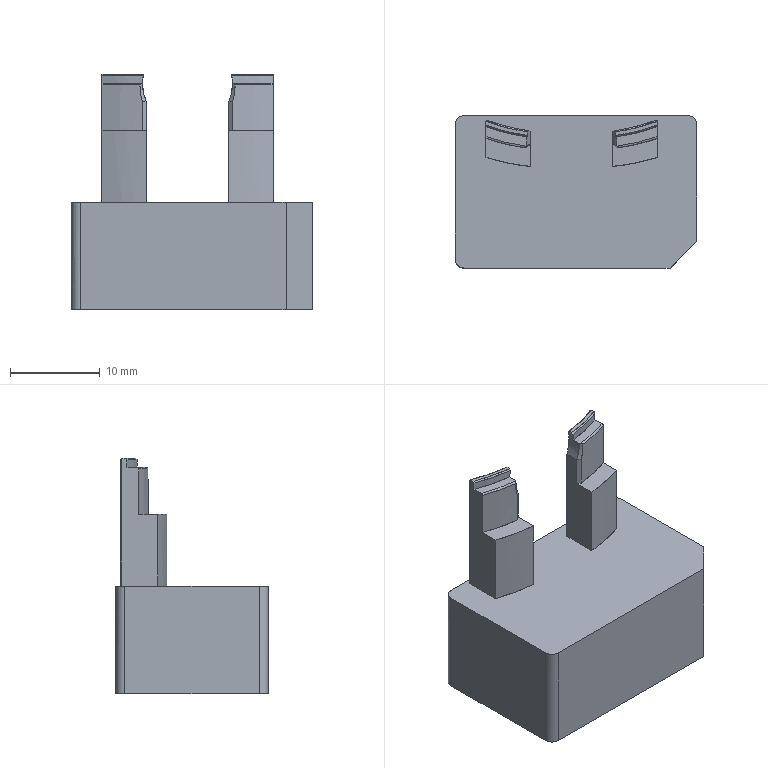NC program | PowerMill | posted by the shop | part box 27 x 17 x 26.255 mm
Lines 1 to 1491 of 169183:
%
G40 G49 G17 G80
( TOOL ID   D10C_1_1_1 )
( TOOL DIA. 10. TIP RAD 0 LENGTH 81.72 )
( Z = -.065 )
T1 M6
T15
G91 G28 Z0
G0 G90 G54
M08
S8000 M3
G0 X0 Y0 M8
G43 Z10.2 H1
X21.28 Y11.28
Z1.135
G1 Z-.065 F6000
X16.28 F10000
X-16.28
Y5.64
X16.28
Y0
X-16.28
Y-5.64
X16.28
Y-11.28
X-16.28
X-21.28
G0 Z10.2
X-.501 Y2.234
Z9.885
X-23.108 Y2.522
Z.76
G1 Z-.44 F6000
X-22.58 F10000
G3 X-17.833 Y7.269 I0 J4.748
G1 Y14.747
G2 X-16.833 Y15.747 I1. J0
G1 X15.832
G2 X16.832 Y14.747 I0 J-1.
G1 Y-10.28
G2 X15.832 Y-11.28 I-1. J0
G1 X-.501
Y-5.336
X-11.502
G2 X-11.889 Y-4.949 I0 J.387
G1 Y-4.312
G2 X-11.528 Y-4.044 I.28 J0
G1 X-11.418 Y-4.077
X-9.556 Y-4.534
X-9.269 Y-4.594
X-8.456 Y-4.751
X-7.639 Y-4.886
X-7.129 Y-4.964
X-6.703 Y-5.019
X-6.274 Y-5.057
X-6.168 Y-5.064
G3 X-3.449 Y-4.906 I.725 J11.016
G1 X-3.329 Y-4.884
G3 X-1.802 Y-4.477 I-1.811 J9.863
G1 X-1.62 Y-4.412
X-1.392 Y-4.327
X-1.167 Y-4.232
X-.975 Y-4.146
G2 X-.025 Y-4.146 I.475 J-1.064
G1 X.167 Y-4.232
X.39 Y-4.326
X.616 Y-4.411
X.799 Y-4.476
G3 X2.328 Y-4.884 I3.341 J9.454
G1 X2.448 Y-4.906
G3 X5.138 Y-5.066 I1.994 J10.86
G1 X5.232 Y-5.06
X5.64 Y-5.025
X6.047 Y-4.972
X7.251 Y-4.788
X9.342 Y-4.355
X10.523 Y-4.035
G2 X10.888 Y-4.314 I.076 J-.279
G1 Y-4.949
G2 X10.501 Y-5.336 I-.387 J0
G1 X-.501
Y-11.28
X-16.833
G2 X-17.833 Y-10.28 I0 J1.
G1 Y7.269
X-15.332 Y7.261
X-15.329 Y8.034
X-15.249 Y8.808
X-15.053 Y9.581
X-14.724 Y10.354
X-14.422 Y10.863
X-14.232 Y11.128
X-13.649 Y11.779
X-12.875 Y12.387
X-12.374 Y12.675
X-12.102 Y12.802
X-11.328 Y13.071
X-10.555 Y13.217
X-9.782 Y13.248
X-9.008 Y13.167
X-8.235 Y12.969
X-7.461 Y12.698
X-6.688 Y12.468
X-5.914 Y12.282
X-4.368 Y11.988
X-4.013 Y11.901
X-3.594 Y11.764
X-2.821 Y11.4
X-2.395 Y11.128
X-2.047 Y10.859
X-1.525 Y10.354
X-1.274 Y10.054
X-.947 Y9.581
G3 X-.053 Y9.581 I.447 J.224
G1 X.273 Y10.053
X.525 Y10.354
X1.046 Y10.859
X1.395 Y11.128
X1.82 Y11.4
X2.593 Y11.764
X3.013 Y11.901
X4.14 Y12.133
X5.687 Y12.46
X7.234 Y12.969
X8.007 Y13.167
X8.781 Y13.248
X9.554 Y13.217
X10.327 Y13.072
X11.101 Y12.803
X11.374 Y12.675
X11.874 Y12.388
X12.515 Y11.901
X13.232 Y11.128
X13.421 Y10.864
X13.724 Y10.354
X14.053 Y9.581
X14.249 Y8.808
X14.329 Y8.034
X14.332 Y7.261
X14.272 Y6.487
X14.195 Y6.068
X14.09 Y5.714
X13.788 Y4.94
X13.329 Y4.167
X12.64 Y3.394
X11.874 Y2.802
X11.563 Y2.62
X11.101 Y2.398
X9.554 Y1.862
X8.007 Y1.436
X6.269 Y1.073
X4.913 Y.875
X4.14 Y.864
X3.367 Y.968
X2.95 Y1.073
X2.593 Y1.193
X1.82 Y1.558
X1.372 Y1.847
X1.046 Y2.1
X.512 Y2.62
X.273 Y2.908
X-.061 Y3.394
G3 X-.939 Y3.394 I-.439 J-.238
G1 X-1.274 Y2.907
X-1.512 Y2.62
X-2.047 Y2.099
X-2.372 Y1.847
X-2.821 Y1.557
X-3.594 Y1.193
X-3.95 Y1.073
X-4.368 Y.968
X-5.141 Y.864
X-5.914 Y.876
X-6.688 Y.978
X-8.235 Y1.26
X-9.782 Y1.636
X-11.328 Y2.114
X-12.102 Y2.398
X-12.561 Y2.62
X-12.875 Y2.802
X-13.649 Y3.399
X-14.325 Y4.167
X-14.789 Y4.94
X-15.091 Y5.714
X-15.196 Y6.072
X-15.272 Y6.487
X-15.332 Y7.261
X-17.833 Y7.269
G0 Z3.435
G1 X-23.108 Y2.522
G0 Z.435
G1 Z-.765 F6000
X-22.58 F10000
G3 X-17.833 Y7.269 I0 J4.748
G1 Y14.747
G2 X-16.833 Y15.747 I1. J0
G1 X15.832
G2 X16.832 Y14.747 I0 J-1.
G1 Y-10.28
G2 X15.832 Y-11.28 I-1. J0
G1 X-.501
Y-5.336
X-11.502
G2 X-11.889 Y-4.949 I0 J.387
G1 Y-4.312
G2 X-11.528 Y-4.044 I.28 J0
G1 X-11.418 Y-4.077
X-9.556 Y-4.534
X-9.269 Y-4.594
X-8.456 Y-4.751
X-7.639 Y-4.886
X-7.129 Y-4.964
X-6.702 Y-5.019
X-6.273 Y-5.057
X-6.167 Y-5.064
G3 X-3.45 Y-4.906 I.724 J11.015
G1 X-3.33 Y-4.884
G3 X-1.802 Y-4.477 I-1.81 J9.864
G1 X-1.619 Y-4.413
X-1.363 Y-4.315
X-1.111 Y-4.207
X-.994 Y-4.153
G2 X-.006 Y-4.153 I.494 J-1.076
G1 X.111 Y-4.207
X.361 Y-4.315
X.616 Y-4.411
X.799 Y-4.476
G3 X2.329 Y-4.884 I3.341 J9.455
G1 X2.449 Y-4.906
G3 X5.137 Y-5.066 I1.993 J10.86
G1 X5.231 Y-5.06
X5.64 Y-5.025
X6.047 Y-4.972
X7.251 Y-4.788
X9.342 Y-4.355
X10.523 Y-4.035
G2 X10.888 Y-4.314 I.076 J-.279
G1 Y-4.949
G2 X10.501 Y-5.336 I-.387 J0
G1 X-.501
Y-11.28
X-16.833
G2 X-17.833 Y-10.28 I0 J1.
G1 Y7.269
X-15.332 Y7.261
X-15.329 Y8.034
X-15.249 Y8.808
X-15.053 Y9.581
X-14.724 Y10.354
X-14.422 Y10.863
X-14.232 Y11.128
X-13.649 Y11.779
X-12.875 Y12.387
X-12.374 Y12.675
X-12.102 Y12.802
X-11.328 Y13.071
X-10.555 Y13.217
X-9.782 Y13.248
X-9.008 Y13.167
X-8.235 Y12.969
X-7.396 Y12.678
X-7.179 Y12.614
X-6.688 Y12.469
X-5.914 Y12.288
X-5.451 Y12.194
X-4.368 Y11.988
X-4.014 Y11.902
X-4.012 Y11.901
X-3.594 Y11.764
X-2.821 Y11.4
X-2.395 Y11.128
X-2.047 Y10.859
X-1.525 Y10.354
X-1.274 Y10.054
X-.947 Y9.581
G3 X-.053 Y9.581 I.447 J.224
G1 X.273 Y10.053
X.525 Y10.354
X1.046 Y10.859
X1.395 Y11.128
X1.82 Y11.4
X2.593 Y11.764
X3.013 Y11.901
X4.14 Y12.133
X5.687 Y12.468
X5.958 Y12.549
X7.23 Y12.968
X7.234 Y12.969
X8.007 Y13.167
X8.781 Y13.248
X9.554 Y13.217
X10.327 Y13.072
X11.101 Y12.803
X11.374 Y12.675
X11.874 Y12.388
X12.515 Y11.901
X13.232 Y11.128
X13.421 Y10.864
X13.724 Y10.354
X14.053 Y9.581
X14.249 Y8.808
X14.329 Y8.034
X14.332 Y7.261
X14.276 Y6.487
X14.195 Y6.068
X14.095 Y5.714
X13.793 Y4.94
X13.334 Y4.167
X12.648 Y3.398
X11.874 Y2.802
X11.567 Y2.62
X11.101 Y2.398
X9.554 Y1.862
X8.007 Y1.436
X6.269 Y1.073
X4.913 Y.875
X4.14 Y.864
X3.367 Y.968
X2.95 Y1.073
X2.593 Y1.193
X1.82 Y1.558
X1.372 Y1.847
X1.046 Y2.1
X.512 Y2.62
X.273 Y2.908
X-.061 Y3.394
G3 X-.939 Y3.394 I-.439 J-.239
G1 X-1.274 Y2.907
X-1.512 Y2.62
X-2.047 Y2.099
X-2.372 Y1.847
X-2.821 Y1.557
X-3.594 Y1.193
X-3.95 Y1.073
X-4.368 Y.968
X-5.141 Y.864
X-5.914 Y.876
X-6.688 Y.978
X-8.235 Y1.26
X-9.782 Y1.636
X-11.328 Y2.114
X-12.102 Y2.398
X-12.564 Y2.62
X-12.875 Y2.802
X-13.643 Y3.394
X-13.646 Y3.396
X-13.649 Y3.399
X-13.755 Y3.519
X-14.33 Y4.167
X-14.794 Y4.94
X-15.096 Y5.714
X-15.196 Y6.072
X-15.277 Y6.487
X-15.332 Y7.261
X-17.833 Y7.269
G0 Z3.11
G1 X-23.108 Y2.522
G0 Z.11
G1 Z-1.09 F6000
X-22.58 F10000
G3 X-17.833 Y7.269 I0 J4.748
G1 Y14.747
G2 X-16.833 Y15.747 I1. J0
G1 X15.832
G2 X16.832 Y14.747 I0 J-1.
G1 Y-10.28
G2 X15.832 Y-11.28 I-1. J0
G1 X-.501
Y-5.336
X-11.502
G2 X-11.889 Y-4.949 I0 J.387
G1 Y-4.312
G2 X-11.528 Y-4.044 I.28 J0
G1 X-11.418 Y-4.077
X-9.556 Y-4.534
X-9.269 Y-4.594
X-8.456 Y-4.751
X-7.638 Y-4.886
X-7.129 Y-4.964
X-6.702 Y-5.019
X-6.273 Y-5.057
X-6.166 Y-5.064
G3 X-3.451 Y-4.906 I.724 J11.015
G1 X-3.331 Y-4.884
G3 X-1.802 Y-4.477 I-1.809 J9.864
G1 X-1.619 Y-4.413
X-1.363 Y-4.315
X-1.111 Y-4.207
X-.994 Y-4.153
G2 X-.006 Y-4.153 I.494 J-1.076
G1 X.111 Y-4.207
X.361 Y-4.315
X.616 Y-4.411
X.799 Y-4.476
G3 X2.331 Y-4.884 I3.341 J9.455
G1 X2.451 Y-4.906
G3 X5.136 Y-5.066 I1.992 J10.859
G1 X5.231 Y-5.06
X5.64 Y-5.025
X6.047 Y-4.972
X7.251 Y-4.788
X9.342 Y-4.355
X10.523 Y-4.035
G2 X10.888 Y-4.314 I.076 J-.279
G1 Y-4.949
G2 X10.501 Y-5.336 I-.387 J0
G1 X-.501
Y-11.28
X-16.833
G2 X-17.833 Y-10.28 I0 J1.
G1 Y6.806
X-15.313 Y6.971
X-15.332 Y7.261
X-15.329 Y8.034
X-15.249 Y8.808
X-15.053 Y9.581
X-14.724 Y10.354
X-14.422 Y10.863
X-14.232 Y11.128
X-13.649 Y11.779
X-12.875 Y12.387
X-12.374 Y12.675
X-12.102 Y12.802
X-11.328 Y13.071
X-10.555 Y13.217
X-9.782 Y13.248
X-9.008 Y13.167
X-8.235 Y12.969
X-7.374 Y12.675
X-6.688 Y12.471
X-5.914 Y12.29
X-5.354 Y12.175
X-4.368 Y11.988
X-4.015 Y11.902
X-4.012 Y11.901
X-3.594 Y11.764
X-2.821 Y11.4
X-2.395 Y11.128
X-2.047 Y10.859
X-1.525 Y10.354
X-1.274 Y10.054
X-.947 Y9.581
G3 X-.053 Y9.581 I.447 J.224
G1 X.273 Y10.053
X.525 Y10.354
X1.046 Y10.859
X1.395 Y11.128
X1.82 Y11.4
X2.593 Y11.764
X3.013 Y11.901
X4.14 Y12.133
X5.687 Y12.471
X6.016 Y12.568
X7.226 Y12.966
X7.234 Y12.969
X8.007 Y13.167
X8.781 Y13.248
X9.554 Y13.217
X10.327 Y13.072
X11.101 Y12.803
X11.374 Y12.675
X11.874 Y12.388
X12.515 Y11.901
X13.232 Y11.128
X13.421 Y10.864
X13.724 Y10.354
X14.053 Y9.581
X14.249 Y8.808
X14.329 Y8.034
X14.332 Y7.261
X14.28 Y6.487
X14.255 Y6.378
X14.195 Y6.068
X14.123 Y5.813
X14.099 Y5.714
X13.797 Y4.94
X13.338 Y4.167
X12.647 Y3.394
X11.874 Y2.802
X11.571 Y2.62
X11.101 Y2.398
X9.554 Y1.862
X8.007 Y1.436
X6.269 Y1.073
X4.913 Y.875
X4.14 Y.864
X3.367 Y.968
X2.95 Y1.073
X2.593 Y1.193
X1.82 Y1.558
X1.372 Y1.847
X1.046 Y2.1
X.512 Y2.62
X.273 Y2.908
X-.061 Y3.394
G3 X-.939 Y3.394 I-.439 J-.239
G1 X-1.274 Y2.907
X-1.512 Y2.62
X-2.047 Y2.099
X-2.372 Y1.847
X-2.821 Y1.557
X-3.594 Y1.193
X-3.95 Y1.073
X-4.368 Y.968
X-5.141 Y.864
X-5.914 Y.876
X-6.688 Y.978
X-8.235 Y1.26
X-9.782 Y1.636
X-11.328 Y2.114
X-12.102 Y2.398
X-12.568 Y2.62
X-12.875 Y2.802
X-12.979 Y2.882
X-13.643 Y3.394
X-13.645 Y3.396
X-13.649 Y3.399
X-14.335 Y4.167
X-14.798 Y4.94
X-15.1 Y5.714
X-15.125 Y5.821
X-15.196 Y6.072
X-15.252 Y6.363
X-15.281 Y6.487
X-15.313 Y6.971
X-17.833 Y6.806
Y7.269
G0 Z2.735
G1 X-23.108 Y2.522
G0 Z-.265
G1 Z-1.465 F6000
X-22.58 F10000
G3 X-17.833 Y7.269 I0 J4.748
G1 Y14.747
G2 X-16.833 Y15.747 I1. J0
G1 X15.832
G2 X16.832 Y14.747 I0 J-1.
G1 Y-5.393
X11.752 Y-5.243
G2 X11.308 Y-5.956 I-.835 J.025
G1 X11.191 Y-6.018
X10.983 Y-6.097
X10.763 Y-6.124
X-11.764
X-11.975 Y-6.099
X-12.175 Y-6.027
X-12.288 Y-5.97
G2 X-11.603 Y-4.427 I.38 J.755
G1 X-11.306 Y-4.542
G3 X-1.746 Y-4.671 I4.954 J12.815
G1 X-1.183 Y-4.471
G2 X.087 Y-4.447 I.67 J-1.884
G1 X1.604 Y-4.924
G3 X10.315 Y-4.562 I3.853 J12.262
G1 X10.601 Y-4.445
G2 X11.752 Y-5.243 I.316 J-.773
G1 X16.832 Y-5.393
Y-10.28
G2 X15.832 Y-11.28 I-1. J0
G1 X-16.833
G2 X-17.833 Y-10.28 I0 J1.
G1 Y5.711
X-15.327 Y5.714
X-15.328 Y7.209
X-15.332 Y7.261
X-15.329 Y8.022
Y8.034
X-15.249 Y8.808
X-15.053 Y9.581
X-14.724 Y10.354
X-14.422 Y10.863
X-14.232 Y11.128
X-13.649 Y11.779
X-12.875 Y12.387
X-12.374 Y12.675
X-12.102 Y12.802
X-11.328 Y13.071
X-10.555 Y13.217
X-9.782 Y13.248
X-9.008 Y13.167
X-8.235 Y12.969
X-7.374 Y12.675
X-6.688 Y12.474
X-5.914 Y12.29
X-5.331 Y12.171
X-4.368 Y11.988
X-4.017 Y11.902
X-4.012 Y11.901
X-3.594 Y11.764
X-2.821 Y11.4
X-2.395 Y11.128
X-2.047 Y10.859
X-1.525 Y10.354
X-1.274 Y10.054
X-.947 Y9.581
G3 X-.053 Y9.581 I.447 J.224
G1 X.273 Y10.053
X.525 Y10.354
X1.046 Y10.859
X1.395 Y11.128
X1.82 Y11.4
X2.593 Y11.764
X3.013 Y11.901
X4.14 Y12.133
X5.687 Y12.473
X6.087 Y12.591
X7.219 Y12.964
X7.234 Y12.969
X8.007 Y13.167
X8.781 Y13.248
X9.554 Y13.217
X10.327 Y13.072
X11.101 Y12.803
X11.374 Y12.675
X11.874 Y12.388
X12.515 Y11.901
X13.232 Y11.128
X13.421 Y10.864
X13.724 Y10.354
X14.053 Y9.581
X14.249 Y8.808
X14.329 Y8.034
Y8.022
X14.332 Y7.261
X14.328 Y7.211
X14.327 Y5.714
X14.236 Y4.94
X14.024 Y4.167
X13.675 Y3.394
X13.421 Y2.98
X13.154 Y2.62
X12.648 Y2.078
X12.382 Y1.847
X11.874 Y1.482
X11.101 Y1.078
X10.327 Y.804
X9.554 Y.564
X8.59 Y.3
X7.234 Y-.01
X5.687 Y-.276
X4.913 Y-.343
X4.14 Y-.307
X3.367 Y-.15
X2.593 Y.138
X2.277 Y.3
X1.82 Y.579
X1.193 Y1.073
X.424 Y1.847
X.273 Y2.042
X-.079 Y2.59
G3 X-.92 Y2.591 I-.421 J-.27
G1 X-1.274 Y2.041
X-1.424 Y1.847
X-2.047 Y1.2
X-2.821 Y.579
X-3.278 Y.3
X-3.594 Y.138
X-4.368 Y-.15
X-5.141 Y-.307
X-5.914 Y-.343
X-6.688 Y-.275
X-8.235 Y-.01
X-9.782 Y.35
X-11.328 Y.805
X-12.09 Y1.073
X-12.875 Y1.482
X-13.382 Y1.847
X-13.649 Y2.079
X-14.154 Y2.62
X-14.422 Y2.981
X-14.675 Y3.394
X-15.024 Y4.167
X-15.196 Y4.752
X-15.327 Y5.714
X-17.833 Y5.711
Y7.269
G0 Z2.36
G1 X-23.108 Y2.522
G0 Z-.64
G1 Z-1.84 F6000
X-22.58 F10000
G3 X-17.833 Y7.269 I0 J4.748
G1 Y14.747
G2 X-16.833 Y15.747 I1. J0
G1 X8.881
X8.781 Y13.248
X9.554 Y13.217
X10.327 Y13.072
X11.101 Y12.803
X11.374 Y12.675
X11.874 Y12.388
X12.515 Y11.901
X13.232 Y11.128
X13.421 Y10.864
X13.724 Y10.354
X14.053 Y9.581
X14.25 Y8.808
X14.329 Y8.034
Y8.01
X14.332 Y7.261
X14.328 Y7.212
X14.327 Y5.714
X14.236 Y4.94
X14.024 Y4.167
X13.675 Y3.394
X13.421 Y2.98
X13.154 Y2.62
X12.648 Y2.078
X12.382 Y1.847
X11.874 Y1.482
X11.101 Y1.078
X10.327 Y.804
X9.554 Y.564
X8.59 Y.3
X7.234 Y-.01
X5.687 Y-.278
X4.913 Y-.35
X4.14 Y-.313
X3.367 Y-.157
X2.593 Y.129
X2.254 Y.3
X1.82 Y.566
X1.183 Y1.073
X.407 Y1.847
X-.087 Y2.568
G3 X-.912 Y2.568 I-.413 J-.282
G1 X-1.406 Y1.847
X-2.047 Y1.193
X-2.821 Y.565
X-3.253 Y.3
X-3.594 Y.129
X-4.368 Y-.158
X-5.141 Y-.313
X-5.914 Y-.35
X-6.688 Y-.278
X-8.235 Y-.01
X-9.782 Y.35
X-11.328 Y.805
X-12.09 Y1.073
X-12.875 Y1.482
X-13.382 Y1.847
X-13.649 Y2.079
X-14.154 Y2.62
X-14.422 Y2.981
X-14.675 Y3.394
X-15.024 Y4.167
X-15.196 Y4.752
X-15.327 Y5.714
X-15.328 Y7.21
X-15.332 Y7.261
X-15.329 Y8.01
Y8.034
X-15.249 Y8.808
X-15.053 Y9.581
X-14.724 Y10.354
X-14.422 Y10.863
X-14.232 Y11.128
X-13.649 Y11.779
X-12.875 Y12.387
X-12.374 Y12.675
X-12.102 Y12.802
X-11.328 Y13.071
X-10.555 Y13.217
X-9.782 Y13.248
X-9.008 Y13.167
X-8.235 Y12.969
X-7.374 Y12.675
X-6.688 Y12.474
X-5.914 Y12.29
X-5.328 Y12.17
X-4.368 Y11.988
X-4.018 Y11.902
X-4.012 Y11.901
X-3.594 Y11.764
X-2.821 Y11.4
X-2.395 Y11.128
X-2.047 Y10.859
X-1.525 Y10.354
X-1.274 Y10.054
X-.947 Y9.581
G3 X-.053 Y9.581 I.447 J.224
G1 X.273 Y10.053
X.525 Y10.354
X1.046 Y10.859
X1.395 Y11.128
X1.82 Y11.4
X2.593 Y11.764
X3.012 Y11.901
X4.14 Y12.133
X5.687 Y12.473
X7.234 Y12.969
X8.007 Y13.167
X8.781 Y13.248
X8.881 Y15.747
X15.832
G2 X16.832 Y14.747 I0 J-1.
G1 Y-4.75
X11.747 Y-5.141
G2 X11.422 Y-5.862 I-.821 J-.063
G1 X11.317 Y-5.941
G2 X10.775 Y-6.123 I-.542 J.718
G1 X-11.776
G2 X-12.311 Y-5.946 I0 J.9
G1 X-12.413 Y-5.871
G2 X-11.612 Y-4.427 I.496 J.669
G1 X-11.32 Y-4.542
G3 X-2.187 Y-4.822 I4.957 J12.58
G1 X-1.094 Y-4.468
G2 X.135 Y-4.466 I.618 J-1.902
G1 X1.444 Y-4.887
G3 X10.005 Y-4.672 I3.973 J12.366
G1 X10.635 Y-4.434
G2 X11.747 Y-5.141 I.291 J-.771
G1 X16.832 Y-4.75
Y-10.28
G2 X15.832 Y-11.28 I-1. J0
G1 X-16.833
G2 X-17.833 Y-10.28 I0 J1.
G1 Y7.269
G0 Z1.985
G1 X-23.108 Y2.522
G0 Z-1.015
G1 Z-2.215 F6000
X-22.58 F10000
G3 X-17.833 Y7.269 I0 J4.748
G1 Y14.747
G2 X-16.833 Y15.747 I1. J0
G1 X8.881
X8.781 Y13.248
X9.554 Y13.217
X10.327 Y13.072
X11.101 Y12.803
X11.374 Y12.675
X11.874 Y12.388
X12.515 Y11.901
X13.232 Y11.128
X13.421 Y10.864
X13.724 Y10.354
X14.053 Y9.581
X14.25 Y8.808
X14.329 Y8.034
Y7.997
X14.332 Y7.261
X14.328 Y7.213
X14.327 Y5.714
X14.236 Y4.94
X14.024 Y4.167
X13.675 Y3.394
X13.421 Y2.98
X13.154 Y2.62
X12.648 Y2.078
X12.382 Y1.847
X11.874 Y1.482
X11.101 Y1.078
X10.327 Y.804
X9.554 Y.564
X8.59 Y.3
X7.234 Y-.01
X5.687 Y-.278
X4.913 Y-.356
X4.14 Y-.322
X3.367 Y-.17
X2.593 Y.109
X2.211 Y.3
X1.82 Y.539
X1.14 Y1.073
X.353 Y1.847
X-.087 Y2.486
G3 X-.913 Y2.482 I-.412 J-.283
G1 X-1.274 Y1.946
X-2.047 Y1.151
X-2.821 Y.539
X-3.212 Y.3
X-3.594 Y.108
X-4.368 Y-.17
X-4.843 Y-.263
X-3.988 Y-5.283
G3 X-1.608 Y-4.656 I-2.325 J13.659
G1 X-1.194 Y-4.507
G2 X.077 Y-4.478 I.679 J-1.881
G1 X1.588 Y-4.946
G3 X10.342 Y-4.556 I3.834 J12.374
G1 X10.625 Y-4.44
G2 X11.505 Y-5.771 I.309 J-.753
G1 X11.41 Y-5.865
G2 X10.787 Y-6.122 I-.623 J.631
G1 X-11.751 Y-6.136
G2 X-12.411 Y-5.865 I-.001 J.937
G1 X-12.505 Y-5.773
G2 X-11.629 Y-4.423 I.578 J.584
G1 X-11.335 Y-4.538
G3 X-3.988 Y-5.283 I5.022 J12.913
G1 X-4.843 Y-.263
X-5.141 Y-.322
X-5.914 Y-.356
X-6.688 Y-.278
X-8.235 Y-.01
X-9.782 Y.35
X-11.328 Y.805
X-12.09 Y1.073
X-12.875 Y1.482
X-13.382 Y1.847
X-13.649 Y2.079
X-14.154 Y2.62
X-14.422 Y2.981
X-14.675 Y3.394
X-15.024 Y4.167
X-15.196 Y4.752
X-15.327 Y5.714
X-15.328 Y7.211
X-15.332 Y7.261
X-15.329 Y7.998
Y8.034
X-15.249 Y8.808
X-15.053 Y9.581
X-14.724 Y10.354
X-14.422 Y10.863
X-14.232 Y11.128
X-13.649 Y11.779
X-12.875 Y12.387
X-12.374 Y12.675
X-12.102 Y12.802
X-11.328 Y13.071
X-10.555 Y13.217
X-9.782 Y13.248
X-9.008 Y13.167
X-8.235 Y12.969
X-7.371 Y12.675
X-6.688 Y12.474
X-5.914 Y12.29
X-5.271 Y12.16
X-4.368 Y11.988
X-4.074 Y11.916
X-4.001 Y11.901
X-3.594 Y11.771
X-2.821 Y11.415
X-2.367 Y11.128
X-2.047 Y10.883
X-1.493 Y10.354
X-1.274 Y10.096
X-.913 Y9.581
G3 X-.087 Y9.581 I.413 J.282
G1 X.273 Y10.095
X.493 Y10.354
X1.046 Y10.883
X1.367 Y11.128
X1.82 Y11.414
X2.593 Y11.77
X3.001 Y11.901
X4.14 Y12.133
X5.687 Y12.473
X7.234 Y12.969
X8.007 Y13.167
X8.781 Y13.248
X8.881 Y15.747
X15.832
G2 X16.832 Y14.747 I0 J-1.
G1 Y-10.28
G2 X15.832 Y-11.28 I-1. J0
G1 X-16.833
G2 X-17.833 Y-10.28 I0 J1.
G1 Y7.269
G0 Z1.61
G1 X-23.108 Y2.522
G0 Z-1.39
G1 Z-2.59 F6000
X-22.58 F10000
G3 X-17.833 Y7.269 I0 J4.748
G1 Y14.747
G2 X-16.833 Y15.747 I1. J0
G1 X8.881
X8.781 Y13.248
X9.554 Y13.217
X10.327 Y13.072
X11.101 Y12.803
X11.374 Y12.675
X11.874 Y12.388
X12.515 Y11.901
X13.232 Y11.128
X13.421 Y10.864
X13.724 Y10.354
X14.053 Y9.581
X14.25 Y8.808
X14.329 Y8.034
Y7.985
X14.332 Y7.261
X14.328 Y7.213
X14.327 Y5.714
X14.236 Y4.94
X14.024 Y4.167
X13.675 Y3.394
X13.421 Y2.98
X13.154 Y2.62
X12.648 Y2.078
X12.382 Y1.847
X11.874 Y1.482
X11.101 Y1.078
X10.327 Y.804
X9.554 Y.564
X8.59 Y.3
X7.234 Y-.01
X5.687 Y-.278
X4.913 Y-.362
X4.14 Y-.338
X3.367 Y-.197
X2.593 Y.069
X2.126 Y.3
X1.82 Y.485
X1.06 Y1.073
X.273 Y1.84
X-.089 Y2.362
G3 X-.911 Y2.361 I-.411 J-.285
G1 X-1.267 Y1.847
X-2.047 Y1.083
X-2.821 Y.484
X-3.127 Y.3
X-3.594 Y.069
X-4.368 Y-.198
X-5.141 Y-.337
X-5.914 Y-.362
X-6.688 Y-.278
X-8.235 Y-.01
X-9.782 Y.35
X-11.328 Y.805
X-12.09 Y1.073
X-12.875 Y1.482
X-13.382 Y1.847
X-13.649 Y2.079
X-14.154 Y2.62
X-14.422 Y2.981
X-14.675 Y3.394
X-15.024 Y4.167
X-15.196 Y4.752
X-15.327 Y5.714
X-15.328 Y7.212
X-15.332 Y7.261
X-15.329 Y7.986
Y8.034
X-15.249 Y8.808
X-15.053 Y9.581
X-14.724 Y10.354
X-14.422 Y10.863
X-14.232 Y11.128
X-13.649 Y11.779
X-12.875 Y12.387
X-12.374 Y12.675
X-12.102 Y12.802
X-11.328 Y13.071
X-10.555 Y13.217
X-9.782 Y13.248
X-9.008 Y13.167
X-8.235 Y12.969
X-6.688 Y12.474
X-5.914 Y12.29
X-4.368 Y11.99
X-4.262 Y11.962
X-4.074 Y11.916
X-4.001 Y11.901
X-3.873 Y11.86
X-3.594 Y11.787
X-2.821 Y11.447
X-2.302 Y11.128
X-2.047 Y10.939
X-1.42 Y10.354
X-1.274 Y10.187
X-.905 Y9.677
G3 X-.094 Y9.678 I.405 J.293
G1 X.273 Y10.186
X.421 Y10.354
X1.046 Y10.938
X1.303 Y11.128
X1.82 Y11.447
X2.593 Y11.785
X2.973 Y11.901
X4.14 Y12.133
X5.687 Y12.473
X7.234 Y12.969
X8.007 Y13.167
X8.781 Y13.248
X8.881 Y15.747
X15.832
G2 X16.832 Y14.747 I0 J-1.
G1 Y-10.28
G2 X15.832 Y-11.28 I-1. J0
G1 X-.501
Y-6.135
X-11.764
G2 X-12.493 Y-5.778 I0 J.924
G1 X-12.575 Y-5.673
G2 X-11.642 Y-4.422 I.639 J.497
G1 X-11.349 Y-4.536
G3 X-1.575 Y-4.687 I5.089 J13.038
G1 X-1.188 Y-4.55
G2 X.057 Y-4.519 I.669 J-1.885
G1 X1.588 Y-4.979
G3 X10.354 Y-4.552 I3.78 J12.583
G1 X10.637 Y-4.436
G2 X11.571 Y-5.678 I.305 J-.743
G1 X11.487 Y-5.784
G2 X10.763 Y-6.135 I-.724 J.573
G1 X-.501
Y-11.28
X-16.833
G2 X-17.833 Y-10.28 I0 J1.
G1 Y7.269
G0 Z1.235
G1 X-23.108 Y2.522
G0 Z-1.765
G1 Z-2.965 F6000
X-22.58 F10000
G3 X-17.833 Y7.269 I0 J4.748
G1 Y14.747
G2 X-16.833 Y15.747 I1. J0
G1 X8.881
X8.781 Y13.248
X9.554 Y13.217
X10.327 Y13.072
X11.101 Y12.803
X11.374 Y12.675
X11.874 Y12.388
X12.515 Y11.901
X13.232 Y11.128
X13.421 Y10.864
X13.724 Y10.354
X14.053 Y9.581
X14.25 Y8.808
X14.329 Y8.034
Y7.973
X14.332 Y7.261
X14.328 Y7.214
X14.327 Y5.714
X14.236 Y4.94
X14.024 Y4.167
X13.675 Y3.394
X13.421 Y2.98
X13.154 Y2.62
X12.648 Y2.078
X12.382 Y1.847
X11.874 Y1.482
X11.101 Y1.078
X10.327 Y.804
X9.554 Y.564
X8.59 Y.3
X7.234 Y-.01
X5.687 Y-.278
X4.913 Y-.37
X4.14 Y-.359
X3.367 Y-.234
X2.593 Y.016
X1.82 Y.411
X1.046 Y.985
X.273 Y1.7
X.146 Y1.847
X-.089 Y2.184
G3 X-.911 Y2.184 I-.411 J-.285
G1 X-1.144 Y1.847
X-1.274 Y1.698
X-1.94 Y1.073
X-2.821 Y.41
X-3.594 Y.016
X-4.368 Y-.234
X-5.141 Y-.359
X-5.914 Y-.37
X-6.688 Y-.278
X-8.235 Y-.01
X-9.782 Y.35
X-11.328 Y.805
X-12.09 Y1.073
X-12.875 Y1.482
X-13.382 Y1.847
X-13.649 Y2.079
X-14.154 Y2.62
X-14.422 Y2.981
X-14.675 Y3.394
X-15.024 Y4.167
X-15.196 Y4.752
X-15.327 Y5.714
X-15.328 Y7.213
X-15.332 Y7.261
X-15.329 Y7.974
Y8.034
X-15.249 Y8.808
X-15.053 Y9.581
X-14.724 Y10.354
X-14.422 Y10.863
X-14.232 Y11.128
X-13.649 Y11.779
X-12.875 Y12.387
X-12.374 Y12.675
X-12.102 Y12.802
X-11.328 Y13.071
X-10.555 Y13.217
X-9.782 Y13.248
X-9.008 Y13.167
X-8.235 Y12.969
X-6.688 Y12.474
X-5.914 Y12.29
X-4.368 Y11.99
X-3.594 Y11.804
X-2.821 Y11.489
X-2.047 Y11.014
X-1.312 Y10.354
X-.898 Y9.815
G3 X-.103 Y9.817 I.397 J.304
G1 X.273 Y10.312
X1.046 Y11.013
X1.82 Y11.488
X2.593 Y11.804
X2.938 Y11.901
X4.14 Y12.133
X5.687 Y12.473
X7.234 Y12.969
X8.007 Y13.167
X8.781 Y13.248
X8.881 Y15.747
X15.832
G2 X16.832 Y14.747 I0 J-1.
G1 Y-5.056
X11.742 Y-5.149
G2 X11.629 Y-5.57 I-.79 J-.014
G1 X11.556 Y-5.692
G2 X10.779 Y-6.133 I-.777 J.466
G1 X-11.78
G2 X-12.562 Y-5.683 I0 J.906
G1 X-12.635 Y-5.559
G2 X-11.657 Y-4.421 I.686 J.4
G1 X-11.367 Y-4.536
G3 X-1.84 Y-4.819 I5.155 J13.015
G1 X-1.129 Y-4.585
G2 X.072 Y-4.57 I.625 J-1.9
G1 X1.466 Y-4.99
G3 X10.369 Y-4.549 I3.831 J12.734
G1 X10.65 Y-4.433
G2 X11.742 Y-5.149 I.301 J-.731
G1 X16.832 Y-5.056
Y-10.28
G2 X15.832 Y-11.28 I-1. J0
G1 X-16.833
G2 X-17.833 Y-10.28 I0 J1.
G1 Y7.269
G0 Z.86
G1 X-23.108 Y2.522
G0 Z-2.14
G1 Z-3.34 F6000
X-22.58 F10000
G3 X-17.833 Y7.269 I0 J4.748
G1 Y14.747
G2 X-16.833 Y15.747 I1. J0
G1 X8.881
X8.781 Y13.248
X9.554 Y13.217
X10.327 Y13.072
X11.101 Y12.803
X11.374 Y12.675
X11.874 Y12.388
X12.515 Y11.901
X13.232 Y11.128
X13.421 Y10.864
X13.724 Y10.354
X14.053 Y9.581
X14.25 Y8.808
X14.329 Y8.034
Y7.96
X14.331 Y7.261
X14.328 Y7.215
X14.327 Y5.714
X14.236 Y4.94
X14.024 Y4.167
X13.675 Y3.394
X13.421 Y2.98
X13.154 Y2.62
X12.648 Y2.078
X12.382 Y1.847
X11.874 Y1.482
X11.101 Y1.078
X10.327 Y.804
X9.554 Y.564
X8.59 Y.3
X8.007 Y.158
X7.666 Y.089
X7.234 Y-.01
X6.83 Y-.08
X6.46 Y-.154
X6.124 Y-.202
X5.687 Y-.278
X5.106 Y-.347
X4.913 Y-.374
X4.14
X3.367 Y-.258
X2.593 Y-.02
X1.924 Y.3
X1.046 Y.918
X.273 Y1.603
X.056 Y1.847
X-.088 Y2.056
G3 X-.912 Y2.056 I-.412 J-.283
G1 X-1.056 Y1.847
X-1.274 Y1.602
X-1.853 Y1.073
X-2.821 Y.36
X-3.594 Y-.02
X-4.368 Y-.259
X-5.141 Y-.374
X-5.914
X-6.688 Y-.278
X-8.235 Y-.01
X-9.782 Y.35
X-11.328 Y.805
X-12.09 Y1.073
X-12.875 Y1.482
X-13.382 Y1.847
X-13.649 Y2.079
X-14.154 Y2.62
X-14.422 Y2.981
X-14.675 Y3.394
X-15.024 Y4.167
X-15.196 Y4.752
X-15.327 Y5.714
X-15.328 Y7.213
X-15.332 Y7.261
X-15.329 Y7.962
Y8.034
X-15.249 Y8.808
X-15.053 Y9.581
X-14.724 Y10.354
X-14.422 Y10.863
X-14.232 Y11.128
X-13.649 Y11.779
X-12.875 Y12.387
X-12.374 Y12.675
X-12.102 Y12.802
X-11.328 Y13.071
X-10.555 Y13.217
X-9.782 Y13.248
X-9.008 Y13.167
X-8.235 Y12.969
X-6.688 Y12.474
X-5.914 Y12.29
X-4.368 Y11.99
X-3.594 Y11.815
X-2.821 Y11.516
X-2.147 Y11.128
X-1.274 Y10.386
X-.896 Y9.9
G3 X-.105 Y9.901 I.395 J.307
G1 X.244 Y10.354
X1.046 Y11.058
X1.82 Y11.515
X2.593 Y11.815
X2.918 Y11.901
X4.14 Y12.133
X5.687 Y12.473
X7.234 Y12.969
X8.007 Y13.167
X8.781 Y13.248
X8.881 Y15.747
X15.832
G2 X16.832 Y14.747 I0 J-1.
G1 Y-10.28
G2 X15.832 Y-11.28 I-1. J0
G1 X-.501
Y-6.146
X-11.754
G2 X-12.605 Y-5.611 I0 J.944
G1 X-12.663 Y-5.49
G2 X-11.668 Y-4.42 I.707 J.34
G1 X-11.377 Y-4.534
G3 X-1.894 Y-4.874 I5.222 J13.228
G1 X-1.109 Y-4.627
G2 X.043 Y-4.613 I.599 J-1.908
G1 X1.489 Y-5.029
G3 X10.378 Y-4.545 I3.748 J13.031
G1 X10.66 Y-4.43
G2 X11.658 Y-5.503 I.297 J-.725
G1 X11.599 Y-5.622
G2 X10.753 Y-6.146 I-.845 J.421
G1 X-.501
Y-11.28
X-16.833
G2 X-17.833 Y-10.28 I0 J1.
G1 Y7.269
G0 Z.485
G1 X-23.108 Y2.522
G0 Z-2.515
G1 Z-3.715 F6000
X-22.58 F10000
G3 X-17.833 Y7.269 I0 J4.748
G1 Y14.747
G2 X-16.833 Y15.747 I1. J0
G1 X8.881
X8.781 Y13.248
X9.554 Y13.217
X10.327 Y13.072
X11.101 Y12.803
X11.374 Y12.675
X11.874 Y12.388
X12.515 Y11.901
X13.232 Y11.128
X13.421 Y10.864
X13.724 Y10.354
X14.053 Y9.581
X14.25 Y8.808
X14.329 Y8.034
Y7.948
X14.331 Y7.261
X14.328 Y7.216
X14.327 Y5.714
X14.236 Y4.94
X14.024 Y4.167
X13.675 Y3.394
X13.421 Y2.98
X13.154 Y2.62
X12.648 Y2.078
X12.382 Y1.847
X11.874 Y1.482
X11.101 Y1.078
X10.327 Y.804
X9.554 Y.564
X8.59 Y.3
X8.007 Y.158
X7.664 Y.088
X7.234 Y-.01
X6.833 Y-.079
X6.46 Y-.154
X6.122 Y-.203
X5.687 Y-.278
X5.108 Y-.347
X4.913 Y-.374
X4.14
X3.367 Y-.258
X2.593 Y-.02
X1.924 Y.3
X1.046 Y.918
X.273 Y1.603
X.056 Y1.847
X-.088 Y2.056
G3 X-.912 Y2.056 I-.412 J-.283
G1 X-1.056 Y1.847
X-1.274 Y1.602
X-1.853 Y1.073
X-2.821 Y.36
X-3.594 Y-.02
X-4.368 Y-.259
X-5.141 Y-.374
X-5.914
X-6.688 Y-.278
X-8.235 Y-.01
X-9.782 Y.35
X-11.328 Y.805
X-12.09 Y1.073
X-12.875 Y1.482
X-13.382 Y1.847
X-13.649 Y2.079
X-14.154 Y2.62
X-14.422 Y2.981
X-14.675 Y3.394
X-15.024 Y4.167
X-15.196 Y4.752
X-15.327 Y5.714
X-15.328 Y7.214
X-15.331 Y7.261
X-15.329 Y7.949
Y8.034
X-15.249 Y8.808
X-15.053 Y9.581
X-14.724 Y10.354
X-14.422 Y10.863
X-14.232 Y11.128
X-13.649 Y11.779
X-12.875 Y12.387
X-12.374 Y12.675
X-12.102 Y12.802
X-11.328 Y13.071
X-10.555 Y13.217
X-9.782 Y13.248
X-9.008 Y13.167
X-8.235 Y12.969
X-6.688 Y12.474
X-5.914 Y12.29
X-4.368 Y11.99
X-3.594 Y11.816
X-2.821 Y11.516
X-2.147 Y11.128
X-1.274 Y10.386
X-.896 Y9.9
G3 X-.105 Y9.901 I.395 J.307
G1 X.244 Y10.354
X1.046 Y11.058
X1.82 Y11.515
X2.593 Y11.815